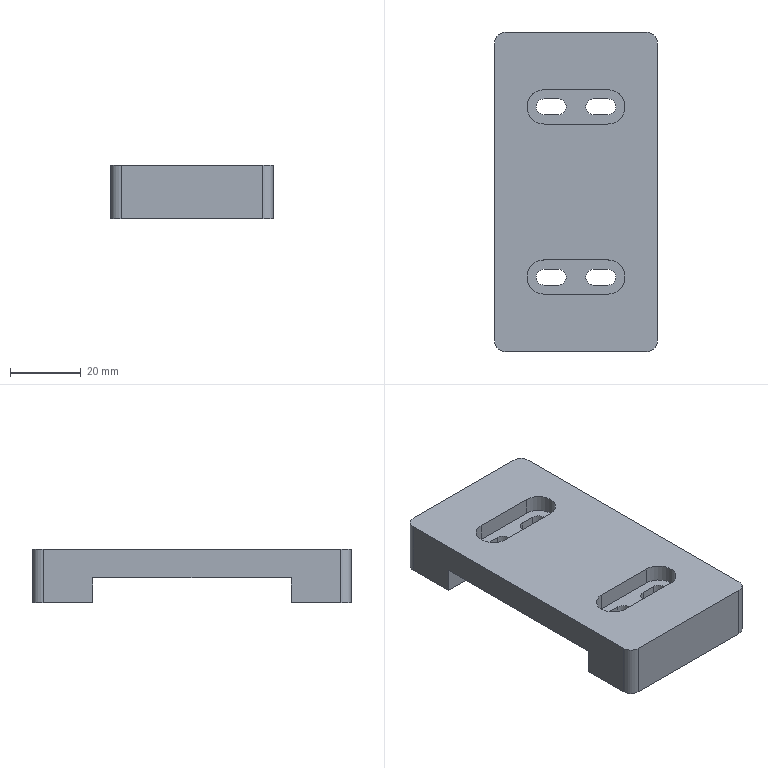Part | STEP file | ROTATION MC_NEW VER-0610_554 | 1 solid | 40 faces | box 46 x 90 x 15 mm | volume 41116 mm3 | plane 24 | cylinder 16 | commonest cylinder face diameters 4.5 x8 6 x4 9.7 x4
STEP:
#1=CARTESIAN_POINT('',(382.531,403.318,-54.091));
#2=VERTEX_POINT('',#1);
#3=CARTESIAN_POINT('',(382.531,403.318,-58.891));
#4=VERTEX_POINT('',#3);
#5=CARTESIAN_POINT('',(382.531,403.318,-54.091));
#6=DIRECTION('',(0.,0.,-1.));
#7=VECTOR('',#6,4.8);
#8=LINE('',#5,#7);
#9=EDGE_CURVE('',#2,#4,#8,.T.);
#10=ORIENTED_EDGE('',*,*,#9,.F.);
#11=CARTESIAN_POINT('',(382.531,393.618,-54.091));
#12=VERTEX_POINT('',#11);
#13=CARTESIAN_POINT('',(382.531,398.468,-54.091));
#14=DIRECTION('',(0.,0.,1.));
#15=DIRECTION('',(-1.,0.,0.));
#16=AXIS2_PLACEMENT_3D('',#13,#14,#15);
#17=CIRCLE('',#16,4.85);
#18=EDGE_CURVE('',#2,#12,#17,.T.);
#19=ORIENTED_EDGE('',*,*,#18,.T.);
#20=CARTESIAN_POINT('',(382.531,393.618,-58.891));
#21=VERTEX_POINT('',#20);
#22=CARTESIAN_POINT('',(382.531,393.618,-58.891));
#23=DIRECTION('',(0.,0.,1.));
#24=VECTOR('',#23,4.8);
#25=LINE('',#22,#24);
#26=EDGE_CURVE('',#21,#12,#25,.T.);
#27=ORIENTED_EDGE('',*,*,#26,.F.);
#28=CARTESIAN_POINT('',(382.531,398.468,-58.891));
#29=DIRECTION('',(0.,0.,-1.));
#30=DIRECTION('',(-1.,0.,0.));
#31=AXIS2_PLACEMENT_3D('',#28,#29,#30);
#32=CIRCLE('',#31,4.85);
#33=EDGE_CURVE('',#21,#4,#32,.T.);
#34=ORIENTED_EDGE('',*,*,#33,.T.);
#35=EDGE_LOOP('',(#10,#19,#27,#34));
#36=FACE_OUTER_BOUND('',#35,.T.);
#37=CARTESIAN_POINT('',(382.531,398.468,-74.091));
#38=DIRECTION('',(0.,0.,1.));
#39=DIRECTION('',(-1.,0.,0.));
#40=AXIS2_PLACEMENT_3D('',#37,#38,#39);
#41=CYLINDRICAL_SURFACE('',#40,4.85);
#42=ADVANCED_FACE('',(#36),#41,.F.);
#43=ORIENTED_EDGE('',*,*,#9,.T.);
#44=CARTESIAN_POINT('',(400.531,403.318,-58.891));
#45=VERTEX_POINT('',#44);
#46=CARTESIAN_POINT('',(382.531,403.318,-58.891));
#47=DIRECTION('',(1.,0.,0.));
#48=VECTOR('',#47,18.);
#49=LINE('',#46,#48);
#50=EDGE_CURVE('',#4,#45,#49,.T.);
#51=ORIENTED_EDGE('',*,*,#50,.T.);
#52=CARTESIAN_POINT('',(400.531,403.318,-54.091));
#53=VERTEX_POINT('',#52);
#54=CARTESIAN_POINT('',(400.531,403.318,-58.891));
#55=DIRECTION('',(0.,0.,1.));
#56=VECTOR('',#55,4.8);
#57=LINE('',#54,#56);
#58=EDGE_CURVE('',#45,#53,#57,.T.);
#59=ORIENTED_EDGE('',*,*,#58,.T.);
#60=CARTESIAN_POINT('',(400.531,403.318,-54.091));
#61=DIRECTION('',(-1.,0.,0.));
#62=VECTOR('',#61,18.);
#63=LINE('',#60,#62);
#64=EDGE_CURVE('',#53,#2,#63,.T.);
#65=ORIENTED_EDGE('',*,*,#64,.T.);
#66=EDGE_LOOP('',(#43,#51,#59,#65));
#67=FACE_OUTER_BOUND('',#66,.T.);
#68=CARTESIAN_POINT('',(384.531,403.318,-74.091));
#69=DIRECTION('',(0.,1.,0.));
#70=DIRECTION('',(0.,0.,1.));
#71=AXIS2_PLACEMENT_3D('',#68,#69,#70);
#72=PLANE('',#71);
#73=ADVANCED_FACE('',(#67),#72,.F.);
#74=ORIENTED_EDGE('',*,*,#26,.T.);
#75=CARTESIAN_POINT('',(400.531,393.618,-54.091));
#76=VERTEX_POINT('',#75);
#77=CARTESIAN_POINT('',(382.531,393.618,-54.091));
#78=DIRECTION('',(1.,0.,0.));
#79=VECTOR('',#78,18.);
#80=LINE('',#77,#79);
#81=EDGE_CURVE('',#12,#76,#80,.T.);
#82=ORIENTED_EDGE('',*,*,#81,.T.);
#83=CARTESIAN_POINT('',(400.531,393.618,-58.891));
#84=VERTEX_POINT('',#83);
#85=CARTESIAN_POINT('',(400.531,393.618,-54.091));
#86=DIRECTION('',(0.,0.,-1.));
#87=VECTOR('',#86,4.8);
#88=LINE('',#85,#87);
#89=EDGE_CURVE('',#76,#84,#88,.T.);
#90=ORIENTED_EDGE('',*,*,#89,.T.);
#91=CARTESIAN_POINT('',(400.531,393.618,-58.891));
#92=DIRECTION('',(-1.,0.,0.));
#93=VECTOR('',#92,18.);
#94=LINE('',#91,#93);
#95=EDGE_CURVE('',#84,#21,#94,.T.);
#96=ORIENTED_EDGE('',*,*,#95,.T.);
#97=EDGE_LOOP('',(#74,#82,#90,#96));
#98=FACE_OUTER_BOUND('',#97,.T.);
#99=CARTESIAN_POINT('',(384.531,393.618,-74.091));
#100=DIRECTION('',(0.,-1.,0.));
#101=DIRECTION('',(0.,0.,-1.));
#102=AXIS2_PLACEMENT_3D('',#99,#100,#101);
#103=PLANE('',#102);
#104=ADVANCED_FACE('',(#98),#103,.F.);
#105=CARTESIAN_POINT('',(382.531,400.718,-58.891));
#106=VERTEX_POINT('',#105);
#107=CARTESIAN_POINT('',(382.531,396.218,-58.891));
#108=VERTEX_POINT('',#107);
#109=CARTESIAN_POINT('',(382.531,398.468,-58.891));
#110=DIRECTION('',(0.,0.,1.));
#111=DIRECTION('',(-1.,0.,0.));
#112=AXIS2_PLACEMENT_3D('',#109,#110,#111);
#113=CIRCLE('',#112,2.25);
#114=EDGE_CURVE('',#106,#108,#113,.T.);
#115=ORIENTED_EDGE('',*,*,#114,.T.);
#116=CARTESIAN_POINT('',(382.531,396.218,-62.091));
#117=VERTEX_POINT('',#116);
#118=CARTESIAN_POINT('',(382.531,396.218,-62.091));
#119=DIRECTION('',(0.,0.,1.));
#120=VECTOR('',#119,3.2);
#121=LINE('',#118,#120);
#122=EDGE_CURVE('',#117,#108,#121,.T.);
#123=ORIENTED_EDGE('',*,*,#122,.F.);
#124=CARTESIAN_POINT('',(382.531,400.718,-62.091));
#125=VERTEX_POINT('',#124);
#126=CARTESIAN_POINT('',(382.531,398.468,-62.091));
#127=DIRECTION('',(0.,0.,1.));
#128=DIRECTION('',(1.,0.,0.));
#129=AXIS2_PLACEMENT_3D('',#126,#127,#128);
#130=CIRCLE('',#129,2.25);
#131=EDGE_CURVE('',#125,#117,#130,.T.);
#132=ORIENTED_EDGE('',*,*,#131,.F.);
#133=CARTESIAN_POINT('',(382.531,400.718,-58.891));
#134=DIRECTION('',(0.,0.,-1.));
#135=VECTOR('',#134,3.2);
#136=LINE('',#133,#135);
#137=EDGE_CURVE('',#106,#125,#136,.T.);
#138=ORIENTED_EDGE('',*,*,#137,.F.);
#139=EDGE_LOOP('',(#115,#123,#132,#138));
#140=FACE_OUTER_BOUND('',#139,.T.);
#141=CARTESIAN_POINT('',(382.531,398.468,-74.091));
#142=DIRECTION('',(0.,0.,1.));
#143=DIRECTION('',(-1.,0.,0.));
#144=AXIS2_PLACEMENT_3D('',#141,#142,#143);
#145=CYLINDRICAL_SURFACE('',#144,2.25);
#146=ADVANCED_FACE('',(#140),#145,.F.);
#147=CARTESIAN_POINT('',(396.531,400.718,-58.891));
#148=VERTEX_POINT('',#147);
#149=CARTESIAN_POINT('',(396.531,396.218,-58.891));
#150=VERTEX_POINT('',#149);
#151=CARTESIAN_POINT('',(396.531,398.468,-58.891));
#152=DIRECTION('',(0.,0.,1.));
#153=DIRECTION('',(-1.,0.,0.));
#154=AXIS2_PLACEMENT_3D('',#151,#152,#153);
#155=CIRCLE('',#154,2.25);
#156=EDGE_CURVE('',#148,#150,#155,.T.);
#157=ORIENTED_EDGE('',*,*,#156,.T.);
#158=CARTESIAN_POINT('',(396.531,396.218,-62.091));
#159=VERTEX_POINT('',#158);
#160=CARTESIAN_POINT('',(396.531,396.218,-62.091));
#161=DIRECTION('',(0.,0.,1.));
#162=VECTOR('',#161,3.2);
#163=LINE('',#160,#162);
#164=EDGE_CURVE('',#159,#150,#163,.T.);
#165=ORIENTED_EDGE('',*,*,#164,.F.);
#166=CARTESIAN_POINT('',(396.531,400.718,-62.091));
#167=VERTEX_POINT('',#166);
#168=CARTESIAN_POINT('',(396.531,398.468,-62.091));
#169=DIRECTION('',(0.,0.,-1.));
#170=DIRECTION('',(1.,0.,0.));
#171=AXIS2_PLACEMENT_3D('',#168,#169,#170);
#172=CIRCLE('',#171,2.25);
#173=EDGE_CURVE('',#159,#167,#172,.T.);
#174=ORIENTED_EDGE('',*,*,#173,.T.);
#175=CARTESIAN_POINT('',(396.531,400.718,-58.891));
#176=DIRECTION('',(0.,0.,-1.));
#177=VECTOR('',#176,3.2);
#178=LINE('',#175,#177);
#179=EDGE_CURVE('',#148,#167,#178,.T.);
#180=ORIENTED_EDGE('',*,*,#179,.F.);
#181=EDGE_LOOP('',(#157,#165,#174,#180));
#182=FACE_OUTER_BOUND('',#181,.T.);
#183=CARTESIAN_POINT('',(396.531,398.468,-74.091));
#184=DIRECTION('',(0.,0.,1.));
#185=DIRECTION('',(-1.,0.,0.));
#186=AXIS2_PLACEMENT_3D('',#183,#184,#185);
#187=CYLINDRICAL_SURFACE('',#186,2.25);
#188=ADVANCED_FACE('',(#182),#187,.F.);
#189=CARTESIAN_POINT('',(386.531,396.218,-58.891));
#190=VERTEX_POINT('',#189);
#191=CARTESIAN_POINT('',(386.531,400.718,-58.891));
#192=VERTEX_POINT('',#191);
#193=CARTESIAN_POINT('',(386.531,398.468,-58.891));
#194=DIRECTION('',(0.,0.,1.));
#195=DIRECTION('',(-1.,0.,0.));
#196=AXIS2_PLACEMENT_3D('',#193,#194,#195);
#197=CIRCLE('',#196,2.25);
#198=EDGE_CURVE('',#190,#192,#197,.T.);
#199=ORIENTED_EDGE('',*,*,#198,.T.);
#200=CARTESIAN_POINT('',(386.531,400.718,-62.091));
#201=VERTEX_POINT('',#200);
#202=CARTESIAN_POINT('',(386.531,400.718,-62.091));
#203=DIRECTION('',(0.,0.,1.));
#204=VECTOR('',#203,3.2);
#205=LINE('',#202,#204);
#206=EDGE_CURVE('',#201,#192,#205,.T.);
#207=ORIENTED_EDGE('',*,*,#206,.F.);
#208=CARTESIAN_POINT('',(386.531,396.218,-62.091));
#209=VERTEX_POINT('',#208);
#210=CARTESIAN_POINT('',(386.531,398.468,-62.091));
#211=DIRECTION('',(0.,0.,-1.));
#212=DIRECTION('',(1.,0.,0.));
#213=AXIS2_PLACEMENT_3D('',#210,#211,#212);
#214=CIRCLE('',#213,2.25);
#215=EDGE_CURVE('',#201,#209,#214,.T.);
#216=ORIENTED_EDGE('',*,*,#215,.T.);
#217=CARTESIAN_POINT('',(386.531,396.218,-58.891));
#218=DIRECTION('',(0.,0.,-1.));
#219=VECTOR('',#218,3.2);
#220=LINE('',#217,#219);
#221=EDGE_CURVE('',#190,#209,#220,.T.);
#222=ORIENTED_EDGE('',*,*,#221,.F.);
#223=EDGE_LOOP('',(#199,#207,#216,#222));
#224=FACE_OUTER_BOUND('',#223,.T.);
#225=CARTESIAN_POINT('',(386.531,398.468,-74.091));
#226=DIRECTION('',(0.,0.,1.));
#227=DIRECTION('',(1.,0.,0.));
#228=AXIS2_PLACEMENT_3D('',#225,#226,#227);
#229=CYLINDRICAL_SURFACE('',#228,2.25);
#230=ADVANCED_FACE('',(#224),#229,.F.);
#231=ORIENTED_EDGE('',*,*,#95,.F.);
#232=CARTESIAN_POINT('',(400.531,398.468,-58.891));
#233=DIRECTION('',(0.,0.,-1.));
#234=DIRECTION('',(-1.,0.,0.));
#235=AXIS2_PLACEMENT_3D('',#232,#233,#234);
#236=CIRCLE('',#235,4.85);
#237=EDGE_CURVE('',#45,#84,#236,.T.);
#238=ORIENTED_EDGE('',*,*,#237,.F.);
#239=ORIENTED_EDGE('',*,*,#50,.F.);
#240=ORIENTED_EDGE('',*,*,#33,.F.);
#241=EDGE_LOOP('',(#231,#238,#239,#240));
#242=FACE_OUTER_BOUND('',#241,.T.);
#243=CARTESIAN_POINT('',(382.531,396.218,-58.891));
#244=DIRECTION('',(1.,0.,0.));
#245=VECTOR('',#244,4.);
#246=LINE('',#243,#245);
#247=EDGE_CURVE('',#108,#190,#246,.T.);
#248=ORIENTED_EDGE('',*,*,#247,.F.);
#249=ORIENTED_EDGE('',*,*,#114,.F.);
#250=CARTESIAN_POINT('',(386.531,400.718,-58.891));
#251=DIRECTION('',(-1.,0.,0.));
#252=VECTOR('',#251,4.);
#253=LINE('',#250,#252);
#254=EDGE_CURVE('',#192,#106,#253,.T.);
#255=ORIENTED_EDGE('',*,*,#254,.F.);
#256=ORIENTED_EDGE('',*,*,#198,.F.);
#257=EDGE_LOOP('',(#248,#249,#255,#256));
#258=FACE_BOUND('',#257,.T.);
#259=CARTESIAN_POINT('',(400.531,396.218,-58.891));
#260=VERTEX_POINT('',#259);
#261=CARTESIAN_POINT('',(396.531,396.218,-58.891));
#262=DIRECTION('',(1.,0.,0.));
#263=VECTOR('',#262,4.);
#264=LINE('',#261,#263);
#265=EDGE_CURVE('',#150,#260,#264,.T.);
#266=ORIENTED_EDGE('',*,*,#265,.F.);
#267=ORIENTED_EDGE('',*,*,#156,.F.);
#268=CARTESIAN_POINT('',(400.531,400.718,-58.891));
#269=VERTEX_POINT('',#268);
#270=CARTESIAN_POINT('',(400.531,400.718,-58.891));
#271=DIRECTION('',(-1.,0.,0.));
#272=VECTOR('',#271,4.);
#273=LINE('',#270,#272);
#274=EDGE_CURVE('',#269,#148,#273,.T.);
#275=ORIENTED_EDGE('',*,*,#274,.F.);
#276=CARTESIAN_POINT('',(400.531,398.468,-58.891));
#277=DIRECTION('',(0.,0.,1.));
#278=DIRECTION('',(-1.,0.,0.));
#279=AXIS2_PLACEMENT_3D('',#276,#277,#278);
#280=CIRCLE('',#279,2.25);
#281=EDGE_CURVE('',#260,#269,#280,.T.);
#282=ORIENTED_EDGE('',*,*,#281,.F.);
#283=EDGE_LOOP('',(#266,#267,#275,#282));
#284=FACE_BOUND('',#283,.T.);
#285=CARTESIAN_POINT('',(391.531,422.468,-58.891));
#286=DIRECTION('',(0.,0.,1.));
#287=DIRECTION('',(1.,0.,0.));
#288=AXIS2_PLACEMENT_3D('',#285,#286,#287);
#289=PLANE('',#288);
#290=ADVANCED_FACE('',(#242,#258,#284),#289,.T.);
#291=ORIENTED_EDGE('',*,*,#254,.T.);
#292=ORIENTED_EDGE('',*,*,#137,.T.);
#293=CARTESIAN_POINT('',(382.531,400.718,-62.091));
#294=DIRECTION('',(1.,0.,0.));
#295=VECTOR('',#294,4.);
#296=LINE('',#293,#295);
#297=EDGE_CURVE('',#125,#201,#296,.T.);
#298=ORIENTED_EDGE('',*,*,#297,.T.);
#299=ORIENTED_EDGE('',*,*,#206,.T.);
#300=EDGE_LOOP('',(#291,#292,#298,#299));
#301=FACE_OUTER_BOUND('',#300,.T.);
#302=CARTESIAN_POINT('',(384.531,400.718,-74.091));
#303=DIRECTION('',(0.,1.,0.));
#304=DIRECTION('',(0.,0.,1.));
#305=AXIS2_PLACEMENT_3D('',#302,#303,#304);
#306=PLANE('',#305);
#307=ADVANCED_FACE('',(#301),#306,.F.);
#308=ORIENTED_EDGE('',*,*,#247,.T.);
#309=ORIENTED_EDGE('',*,*,#221,.T.);
#310=CARTESIAN_POINT('',(386.531,396.218,-62.091));
#311=DIRECTION('',(-1.,0.,0.));
#312=VECTOR('',#311,4.);
#313=LINE('',#310,#312);
#314=EDGE_CURVE('',#209,#117,#313,.T.);
#315=ORIENTED_EDGE('',*,*,#314,.T.);
#316=ORIENTED_EDGE('',*,*,#122,.T.);
#317=EDGE_LOOP('',(#308,#309,#315,#316));
#318=FACE_OUTER_BOUND('',#317,.T.);
#319=CARTESIAN_POINT('',(384.531,396.218,-74.091));
#320=DIRECTION('',(0.,-1.,0.));
#321=DIRECTION('',(0.,0.,-1.));
#322=AXIS2_PLACEMENT_3D('',#319,#320,#321);
#323=PLANE('',#322);
#324=ADVANCED_FACE('',(#318),#323,.F.);
#325=ORIENTED_EDGE('',*,*,#265,.T.);
#326=CARTESIAN_POINT('',(400.531,396.218,-62.091));
#327=VERTEX_POINT('',#326);
#328=CARTESIAN_POINT('',(400.531,396.218,-58.891));
#329=DIRECTION('',(0.,0.,-1.));
#330=VECTOR('',#329,3.2);
#331=LINE('',#328,#330);
#332=EDGE_CURVE('',#260,#327,#331,.T.);
#333=ORIENTED_EDGE('',*,*,#332,.T.);
#334=CARTESIAN_POINT('',(400.531,396.218,-62.091));
#335=DIRECTION('',(-1.,0.,0.));
#336=VECTOR('',#335,4.);
#337=LINE('',#334,#336);
#338=EDGE_CURVE('',#327,#159,#337,.T.);
#339=ORIENTED_EDGE('',*,*,#338,.T.);
#340=ORIENTED_EDGE('',*,*,#164,.T.);
#341=EDGE_LOOP('',(#325,#333,#339,#340));
#342=FACE_OUTER_BOUND('',#341,.T.);
#343=CARTESIAN_POINT('',(398.531,396.218,-74.091));
#344=DIRECTION('',(0.,-1.,0.));
#345=DIRECTION('',(0.,0.,-1.));
#346=AXIS2_PLACEMENT_3D('',#343,#344,#345);
#347=PLANE('',#346);
#348=ADVANCED_FACE('',(#342),#347,.F.);
#349=ORIENTED_EDGE('',*,*,#274,.T.);
#350=ORIENTED_EDGE('',*,*,#179,.T.);
#351=CARTESIAN_POINT('',(400.531,400.718,-62.091));
#352=VERTEX_POINT('',#351);
#353=CARTESIAN_POINT('',(396.531,400.718,-62.091));
#354=DIRECTION('',(1.,0.,0.));
#355=VECTOR('',#354,4.);
#356=LINE('',#353,#355);
#357=EDGE_CURVE('',#167,#352,#356,.T.);
#358=ORIENTED_EDGE('',*,*,#357,.T.);
#359=CARTESIAN_POINT('',(400.531,400.718,-62.091));
#360=DIRECTION('',(0.,0.,1.));
#361=VECTOR('',#360,3.2);
#362=LINE('',#359,#361);
#363=EDGE_CURVE('',#352,#269,#362,.T.);
#364=ORIENTED_EDGE('',*,*,#363,.T.);
#365=EDGE_LOOP('',(#349,#350,#358,#364));
#366=FACE_OUTER_BOUND('',#365,.T.);
#367=CARTESIAN_POINT('',(398.531,400.718,-74.091));
#368=DIRECTION('',(0.,1.,0.));
#369=DIRECTION('',(0.,0.,1.));
#370=AXIS2_PLACEMENT_3D('',#367,#368,#369);
#371=PLANE('',#370);
#372=ADVANCED_FACE('',(#366),#371,.F.);
#373=ORIENTED_EDGE('',*,*,#281,.T.);
#374=ORIENTED_EDGE('',*,*,#363,.F.);
#375=CARTESIAN_POINT('',(400.531,398.468,-62.091));
#376=DIRECTION('',(0.,0.,-1.));
#377=DIRECTION('',(1.,0.,0.));
#378=AXIS2_PLACEMENT_3D('',#375,#376,#377);
#379=CIRCLE('',#378,2.25);
#380=EDGE_CURVE('',#352,#327,#379,.T.);
#381=ORIENTED_EDGE('',*,*,#380,.T.);
#382=ORIENTED_EDGE('',*,*,#332,.F.);
#383=EDGE_LOOP('',(#373,#374,#381,#382));
#384=FACE_OUTER_BOUND('',#383,.T.);
#385=CARTESIAN_POINT('',(400.531,398.468,-74.091));
#386=DIRECTION('',(0.,0.,1.));
#387=DIRECTION('',(1.,0.,0.));
#388=AXIS2_PLACEMENT_3D('',#385,#386,#387);
#389=CYLINDRICAL_SURFACE('',#388,2.25);
#390=ADVANCED_FACE('',(#384),#389,.F.);
#391=ORIENTED_EDGE('',*,*,#89,.F.);
#392=CARTESIAN_POINT('',(400.531,398.468,-54.091));
#393=DIRECTION('',(0.,0.,1.));
#394=DIRECTION('',(-1.,0.,0.));
#395=AXIS2_PLACEMENT_3D('',#392,#393,#394);
#396=CIRCLE('',#395,4.85);
#397=EDGE_CURVE('',#76,#53,#396,.T.);
#398=ORIENTED_EDGE('',*,*,#397,.T.);
#399=ORIENTED_EDGE('',*,*,#58,.F.);
#400=ORIENTED_EDGE('',*,*,#237,.T.);
#401=EDGE_LOOP('',(#391,#398,#399,#400));
#402=FACE_OUTER_BOUND('',#401,.T.);
#403=CARTESIAN_POINT('',(400.531,398.468,-74.091));
#404=DIRECTION('',(0.,0.,1.));
#405=DIRECTION('',(1.,0.,0.));
#406=AXIS2_PLACEMENT_3D('',#403,#404,#405);
#407=CYLINDRICAL_SURFACE('',#406,4.85);
#408=ADVANCED_FACE('',(#402),#407,.F.);
#409=CARTESIAN_POINT('',(368.531,380.468,-54.091));
#410=VERTEX_POINT('',#409);
#411=CARTESIAN_POINT('',(371.531,377.468,-54.091));
#412=VERTEX_POINT('',#411);
#413=CARTESIAN_POINT('',(371.531,380.468,-54.091));
#414=DIRECTION('',(0.,0.,1.));
#415=DIRECTION('',(-0.7071,-0.7071,0.));
#416=AXIS2_PLACEMENT_3D('',#413,#414,#415);
#417=CIRCLE('',#416,3.);
#418=EDGE_CURVE('',#410,#412,#417,.T.);
#419=ORIENTED_EDGE('',*,*,#418,.T.);
#420=CARTESIAN_POINT('',(411.531,377.468,-54.091));
#421=VERTEX_POINT('',#420);
#422=CARTESIAN_POINT('',(371.531,377.468,-54.091));
#423=DIRECTION('',(1.,0.,0.));
#424=VECTOR('',#423,40.);
#425=LINE('',#422,#424);
#426=EDGE_CURVE('',#412,#421,#425,.T.);
#427=ORIENTED_EDGE('',*,*,#426,.T.);
#428=CARTESIAN_POINT('',(414.531,380.468,-54.091));
#429=VERTEX_POINT('',#428);
#430=CARTESIAN_POINT('',(411.531,380.468,-54.091));
#431=DIRECTION('',(0.,0.,1.));
#432=DIRECTION('',(0.,-1.,0.));
#433=AXIS2_PLACEMENT_3D('',#430,#431,#432);
#434=CIRCLE('',#433,3.);
#435=EDGE_CURVE('',#421,#429,#434,.T.);
#436=ORIENTED_EDGE('',*,*,#435,.T.);
#437=CARTESIAN_POINT('',(414.531,464.468,-54.091));
#438=VERTEX_POINT('',#437);
#439=CARTESIAN_POINT('',(414.531,380.468,-54.091));
#440=DIRECTION('',(0.,1.,0.));
#441=VECTOR('',#440,84.);
#442=LINE('',#439,#441);
#443=EDGE_CURVE('',#429,#438,#442,.T.);
#444=ORIENTED_EDGE('',*,*,#443,.T.);
#445=CARTESIAN_POINT('',(411.531,467.468,-54.091));
#446=VERTEX_POINT('',#445);
#447=CARTESIAN_POINT('',(411.531,464.468,-54.091));
#448=DIRECTION('',(0.,0.,1.));
#449=DIRECTION('',(1.,0.,0.));
#450=AXIS2_PLACEMENT_3D('',#447,#448,#449);
#451=CIRCLE('',#450,3.);
#452=EDGE_CURVE('',#438,#446,#451,.T.);
#453=ORIENTED_EDGE('',*,*,#452,.T.);
#454=CARTESIAN_POINT('',(371.531,467.468,-54.091));
#455=VERTEX_POINT('',#454);
#456=CARTESIAN_POINT('',(411.531,467.468,-54.091));
#457=DIRECTION('',(-1.,0.,0.));
#458=VECTOR('',#457,40.);
#459=LINE('',#456,#458);
#460=EDGE_CURVE('',#446,#455,#459,.T.);
#461=ORIENTED_EDGE('',*,*,#460,.T.);
#462=CARTESIAN_POINT('',(368.531,464.468,-54.091));
#463=VERTEX_POINT('',#462);
#464=CARTESIAN_POINT('',(371.531,464.468,-54.091));
#465=DIRECTION('',(0.,0.,1.));
#466=DIRECTION('',(0.,1.,0.));
#467=AXIS2_PLACEMENT_3D('',#464,#465,#466);
#468=CIRCLE('',#467,3.);
#469=EDGE_CURVE('',#455,#463,#468,.T.);
#470=ORIENTED_EDGE('',*,*,#469,.T.);
#471=CARTESIAN_POINT('',(368.531,464.468,-54.091));
#472=DIRECTION('',(0.,-1.,0.));
#473=VECTOR('',#472,84.);
#474=LINE('',#471,#473);
#475=EDGE_CURVE('',#463,#410,#474,.T.);
#476=ORIENTED_EDGE('',*,*,#475,.T.);
#477=EDGE_LOOP('',(#419,#427,#436,#444,#453,#461,#470,#476));
#478=FACE_OUTER_BOUND('',#477,.T.);
#479=CARTESIAN_POINT('',(382.531,441.618,-54.091));
#480=VERTEX_POINT('',#479);
#481=CARTESIAN_POINT('',(400.531,441.618,-54.091));
#482=VERTEX_POINT('',#481);
#483=CARTESIAN_POINT('',(382.531,441.618,-54.091));
#484=DIRECTION('',(1.,0.,0.));
#485=VECTOR('',#484,18.);
#486=LINE('',#483,#485);
#487=EDGE_CURVE('',#480,#482,#486,.T.);
#488=ORIENTED_EDGE('',*,*,#487,.F.);
#489=CARTESIAN_POINT('',(382.531,451.318,-54.091));
#490=VERTEX_POINT('',#489);
#491=CARTESIAN_POINT('',(382.531,446.468,-54.091));
#492=DIRECTION('',(0.,0.,-1.));
#493=DIRECTION('',(-1.,0.,0.));
#494=AXIS2_PLACEMENT_3D('',#491,#492,#493);
#495=CIRCLE('',#494,4.85);
#496=EDGE_CURVE('',#480,#490,#495,.T.);
#497=ORIENTED_EDGE('',*,*,#496,.T.);
#498=CARTESIAN_POINT('',(400.531,451.318,-54.091));
#499=VERTEX_POINT('',#498);
#500=CARTESIAN_POINT('',(400.531,451.318,-54.091));
#501=DIRECTION('',(-1.,0.,0.));
#502=VECTOR('',#501,18.);
#503=LINE('',#500,#502);
#504=EDGE_CURVE('',#499,#490,#503,.T.);
#505=ORIENTED_EDGE('',*,*,#504,.F.);
#506=CARTESIAN_POINT('',(400.531,446.468,-54.091));
#507=DIRECTION('',(0.,0.,-1.));
#508=DIRECTION('',(-1.,0.,0.));
#509=AXIS2_PLACEMENT_3D('',#506,#507,#508);
#510=CIRCLE('',#509,4.85);
#511=EDGE_CURVE('',#499,#482,#510,.T.);
#512=ORIENTED_EDGE('',*,*,#511,.T.);
#513=EDGE_LOOP('',(#488,#497,#505,#512));
#514=FACE_BOUND('',#513,.T.);
#515=ORIENTED_EDGE('',*,*,#397,.F.);
#516=ORIENTED_EDGE('',*,*,#81,.F.);
#517=ORIENTED_EDGE('',*,*,#18,.F.);
#518=ORIENTED_EDGE('',*,*,#64,.F.);
#519=EDGE_LOOP('',(#515,#516,#517,#518));
#520=FACE_BOUND('',#519,.T.);
#521=CARTESIAN_POINT('',(389.531,422.468,-54.091));
#522=DIRECTION('',(0.,0.,1.));
#523=DIRECTION('',(1.,0.,0.));
#524=AXIS2_PLACEMENT_3D('',#521,#522,#523);
#525=PLANE('',#524);
#526=ADVANCED_FACE('',(#478,#514,#520),#525,.T.);
#527=CARTESIAN_POINT('',(382.531,441.618,-58.891));
#528=VERTEX_POINT('',#527);
#529=CARTESIAN_POINT('',(382.531,441.618,-58.891));
#530=DIRECTION('',(0.,0.,1.));
#531=VECTOR('',#530,4.8);
#532=LINE('',#529,#531);
#533=EDGE_CURVE('',#528,#480,#532,.T.);
#534=ORIENTED_EDGE('',*,*,#533,.T.);
#535=ORIENTED_EDGE('',*,*,#487,.T.);
#536=CARTESIAN_POINT('',(400.531,441.618,-58.891));
#537=VERTEX_POINT('',#536);
#538=CARTESIAN_POINT('',(400.531,441.618,-54.091));
#539=DIRECTION('',(0.,0.,-1.));
#540=VECTOR('',#539,4.8);
#541=LINE('',#538,#540);
#542=EDGE_CURVE('',#482,#537,#541,.T.);
#543=ORIENTED_EDGE('',*,*,#542,.T.);
#544=CARTESIAN_POINT('',(400.531,441.618,-58.891));
#545=DIRECTION('',(-1.,0.,0.));
#546=VECTOR('',#545,18.);
#547=LINE('',#544,#546);
#548=EDGE_CURVE('',#537,#528,#547,.T.);
#549=ORIENTED_EDGE('',*,*,#548,.T.);
#550=EDGE_LOOP('',(#534,#535,#543,#549));
#551=FACE_OUTER_BOUND('',#550,.T.);
#552=CARTESIAN_POINT('',(384.531,441.618,-74.091));
#553=DIRECTION('',(0.,-1.,0.));
#554=DIRECTION('',(0.,0.,-1.));
#555=AXIS2_PLACEMENT_3D('',#552,#553,#554);
#556=PLANE('',#555);
#557=ADVANCED_FACE('',(#551),#556,.F.);
#558=ORIENTED_EDGE('',*,*,#533,.F.);
#559=CARTESIAN_POINT('',(382.531,451.318,-58.891));
#560=VERTEX_POINT('',#559);
#561=CARTESIAN_POINT('',(382.531,446.468,-58.891));
#562=DIRECTION('',(0.,0.,-1.));
#563=DIRECTION('',(-1.,0.,0.));
#564=AXIS2_PLACEMENT_3D('',#561,#562,#563);
#565=CIRCLE('',#564,4.85);
#566=EDGE_CURVE('',#528,#560,#565,.T.);
#567=ORIENTED_EDGE('',*,*,#566,.T.);
#568=CARTESIAN_POINT('',(382.531,451.318,-54.091));
#569=DIRECTION('',(0.,0.,-1.));
#570=VECTOR('',#569,4.8);
#571=LINE('',#568,#570);
#572=EDGE_CURVE('',#490,#560,#571,.T.);
#573=ORIENTED_EDGE('',*,*,#572,.F.);
#574=ORIENTED_EDGE('',*,*,#496,.F.);
#575=EDGE_LOOP('',(#558,#567,#573,#574));
#576=FACE_OUTER_BOUND('',#575,.T.);
#577=CARTESIAN_POINT('',(382.531,446.468,-74.091));
#578=DIRECTION('',(0.,0.,1.));
#579=DIRECTION('',(-1.,0.,0.));
#580=AXIS2_PLACEMENT_3D('',#577,#578,#579);
#581=CYLINDRICAL_SURFACE('',#580,4.85);
#582=ADVANCED_FACE('',(#576),#581,.F.);
#583=ORIENTED_EDGE('',*,*,#572,.T.);
#584=CARTESIAN_POINT('',(400.531,451.318,-58.891));
#585=VERTEX_POINT('',#584);
#586=CARTESIAN_POINT('',(382.531,451.318,-58.891));
#587=DIRECTION('',(1.,0.,0.));
#588=VECTOR('',#587,18.);
#589=LINE('',#586,#588);
#590=EDGE_CURVE('',#560,#585,#589,.T.);
#591=ORIENTED_EDGE('',*,*,#590,.T.);
#592=CARTESIAN_POINT('',(400.531,451.318,-58.891));
#593=DIRECTION('',(0.,0.,1.));
#594=VECTOR('',#593,4.8);
#595=LINE('',#592,#594);
#596=EDGE_CURVE('',#585,#499,#595,.T.);
#597=ORIENTED_EDGE('',*,*,#596,.T.);
#598=ORIENTED_EDGE('',*,*,#504,.T.);
#599=EDGE_LOOP('',(#583,#591,#597,#598));
#600=FACE_OUTER_BOUND('',#599,.T.);
#601=CARTESIAN_POINT('',(384.531,451.318,-74.091));
#602=DIRECTION('',(0.,1.,0.));
#603=DIRECTION('',(0.,0.,1.));
#604=AXIS2_PLACEMENT_3D('',#601,#602,#603);
#605=PLANE('',#604);
#606=ADVANCED_FACE('',(#600),#605,.F.);
#607=ORIENTED_EDGE('',*,*,#596,.F.);
#608=CARTESIAN_POINT('',(400.531,446.468,-58.891));
#609=DIRECTION('',(0.,0.,-1.));
#610=DIRECTION('',(-1.,0.,0.));
#611=AXIS2_PLACEMENT_3D('',#608,#609,#610);
#612=CIRCLE('',#611,4.85);
#613=EDGE_CURVE('',#585,#537,#612,.T.);
#614=ORIENTED_EDGE('',*,*,#613,.T.);
#615=ORIENTED_EDGE('',*,*,#542,.F.);
#616=ORIENTED_EDGE('',*,*,#511,.F.);
#617=EDGE_LOOP('',(#607,#614,#615,#616));
#618=FACE_OUTER_BOUND('',#617,.T.);
#619=CARTESIAN_POINT('',(400.531,446.468,-74.091));
#620=DIRECTION('',(0.,0.,1.));
#621=DIRECTION('',(1.,0.,0.));
#622=AXIS2_PLACEMENT_3D('',#619,#620,#621);
#623=CYLINDRICAL_SURFACE('',#622,4.85);
#624=ADVANCED_FACE('',(#618),#623,.F.);
#625=CARTESIAN_POINT('',(368.531,380.468,-69.091));
#626=VERTEX_POINT('',#625);
#627=CARTESIAN_POINT('',(368.531,380.468,-54.091));
#628=DIRECTION('',(0.,0.,-1.));
#629=VECTOR('',#628,15.);
#630=LINE('',#627,#629);
#631=EDGE_CURVE('',#410,#626,#630,.T.);
#632=ORIENTED_EDGE('',*,*,#631,.T.);
#633=CARTESIAN_POINT('',(371.531,377.468,-69.091));
#634=VERTEX_POINT('',#633);
#635=CARTESIAN_POINT('',(371.531,380.468,-69.091));
#636=DIRECTION('',(0.,0.,-1.));
#637=DIRECTION('',(0.,-1.,0.));
#638=AXIS2_PLACEMENT_3D('',#635,#636,#637);
#639=CIRCLE('',#638,3.);
#640=EDGE_CURVE('',#634,#626,#639,.T.);
#641=ORIENTED_EDGE('',*,*,#640,.F.);
#642=CARTESIAN_POINT('',(371.531,377.468,-69.091));
#643=DIRECTION('',(0.,0.,1.));
#644=VECTOR('',#643,15.);
#645=LINE('',#642,#644);
#646=EDGE_CURVE('',#634,#412,#645,.T.);
#647=ORIENTED_EDGE('',*,*,#646,.T.);
#648=ORIENTED_EDGE('',*,*,#418,.F.);
#649=EDGE_LOOP('',(#632,#641,#647,#648));
#650=FACE_OUTER_BOUND('',#649,.T.);
#651=CARTESIAN_POINT('',(371.531,380.468,-67.091));
#652=DIRECTION('',(0.,0.,-1.));
#653=DIRECTION('',(-0.7071,-0.7071,0.));
#654=AXIS2_PLACEMENT_3D('',#651,#652,#653);
#655=CYLINDRICAL_SURFACE('',#654,3.);
#656=ADVANCED_FACE('',(#650),#655,.T.);
#657=ORIENTED_EDGE('',*,*,#646,.F.);
#658=CARTESIAN_POINT('',(411.531,377.468,-69.091));
#659=VERTEX_POINT('',#658);
#660=CARTESIAN_POINT('',(371.531,377.468,-69.091));
#661=DIRECTION('',(1.,0.,0.));
#662=VECTOR('',#661,40.);
#663=LINE('',#660,#662);
#664=EDGE_CURVE('',#634,#659,#663,.T.);
#665=ORIENTED_EDGE('',*,*,#664,.T.);
#666=CARTESIAN_POINT('',(411.531,377.468,-54.091));
#667=DIRECTION('',(0.,0.,-1.));
#668=VECTOR('',#667,15.);
#669=LINE('',#666,#668);
#670=EDGE_CURVE('',#421,#659,#669,.T.);
#671=ORIENTED_EDGE('',*,*,#670,.F.);
#672=ORIENTED_EDGE('',*,*,#426,.F.);
#673=EDGE_LOOP('',(#657,#665,#671,#672));
#674=FACE_OUTER_BOUND('',#673,.T.);
#675=CARTESIAN_POINT('',(390.531,377.468,-67.091));
#676=DIRECTION('',(0.,-1.,0.));
#677=DIRECTION('',(0.,0.,-1.));
#678=AXIS2_PLACEMENT_3D('',#675,#676,#677);
#679=PLANE('',#678);
#680=ADVANCED_FACE('',(#674),#679,.T.);
#681=ORIENTED_EDGE('',*,*,#670,.T.);
#682=CARTESIAN_POINT('',(414.531,380.468,-69.091));
#683=VERTEX_POINT('',#682);
#684=CARTESIAN_POINT('',(411.531,380.468,-69.091));
#685=DIRECTION('',(0.,0.,-1.));
#686=DIRECTION('',(1.,0.,0.));
#687=AXIS2_PLACEMENT_3D('',#684,#685,#686);
#688=CIRCLE('',#687,3.);
#689=EDGE_CURVE('',#683,#659,#688,.T.);
#690=ORIENTED_EDGE('',*,*,#689,.F.);
#691=CARTESIAN_POINT('',(414.531,380.468,-69.091));
#692=DIRECTION('',(0.,0.,1.));
#693=VECTOR('',#692,15.);
#694=LINE('',#691,#693);
#695=EDGE_CURVE('',#683,#429,#694,.T.);
#696=ORIENTED_EDGE('',*,*,#695,.T.);
#697=ORIENTED_EDGE('',*,*,#435,.F.);
#698=EDGE_LOOP('',(#681,#690,#696,#697));
#699=FACE_OUTER_BOUND('',#698,.T.);
#700=CARTESIAN_POINT('',(411.531,380.468,-67.091));
#701=DIRECTION('',(0.,0.,-1.));
#702=DIRECTION('',(0.7071,-0.7071,0.));
#703=AXIS2_PLACEMENT_3D('',#700,#701,#702);
#704=CYLINDRICAL_SURFACE('',#703,3.);
#705=ADVANCED_FACE('',(#699),#704,.T.);
#706=CARTESIAN_POINT('',(368.531,450.493,-62.091));
#707=VERTEX_POINT('',#706);
#708=CARTESIAN_POINT('',(368.531,394.443,-62.091));
#709=VERTEX_POINT('',#708);
#710=CARTESIAN_POINT('',(368.531,450.493,-62.091));
#711=DIRECTION('',(0.,-1.,0.));
#712=VECTOR('',#711,56.05);
#713=LINE('',#710,#712);
#714=EDGE_CURVE('',#707,#709,#713,.T.);
#715=ORIENTED_EDGE('',*,*,#714,.F.);
#716=CARTESIAN_POINT('',(414.531,450.493,-62.091));
#717=VERTEX_POINT('',#716);
#718=CARTESIAN_POINT('',(414.531,450.493,-62.091));
#719=DIRECTION('',(-1.,0.,0.));
#720=VECTOR('',#719,46.);
#721=LINE('',#718,#720);
#722=EDGE_CURVE('',#717,#707,#721,.T.);
#723=ORIENTED_EDGE('',*,*,#722,.F.);
#724=CARTESIAN_POINT('',(414.531,394.443,-62.091));
#725=VERTEX_POINT('',#724);
#726=CARTESIAN_POINT('',(414.531,394.443,-62.091));
#727=DIRECTION('',(0.,1.,0.));
#728=VECTOR('',#727,56.05);
#729=LINE('',#726,#728);
#730=EDGE_CURVE('',#725,#717,#729,.T.);
#731=ORIENTED_EDGE('',*,*,#730,.F.);
#732=CARTESIAN_POINT('',(368.531,394.443,-62.091));
#733=DIRECTION('',(1.,0.,0.));
#734=VECTOR('',#733,46.);
#735=LINE('',#732,#734);
#736=EDGE_CURVE('',#709,#725,#735,.T.);
#737=ORIENTED_EDGE('',*,*,#736,.F.);
#738=EDGE_LOOP('',(#715,#723,#731,#737));
#739=FACE_OUTER_BOUND('',#738,.T.);
#740=CARTESIAN_POINT('',(400.531,444.218,-62.091));
#741=VERTEX_POINT('',#740);
#742=CARTESIAN_POINT('',(400.531,448.718,-62.091));
#743=VERTEX_POINT('',#742);
#744=CARTESIAN_POINT('',(400.531,446.468,-62.091));
#745=DIRECTION('',(0.,0.,1.));
#746=DIRECTION('',(1.,0.,0.));
#747=AXIS2_PLACEMENT_3D('',#744,#745,#746);
#748=CIRCLE('',#747,2.25);
#749=EDGE_CURVE('',#741,#743,#748,.T.);
#750=ORIENTED_EDGE('',*,*,#749,.T.);
#751=CARTESIAN_POINT('',(396.531,448.718,-62.091));
#752=VERTEX_POINT('',#751);
#753=CARTESIAN_POINT('',(396.531,448.718,-62.091));
#754=DIRECTION('',(1.,0.,0.));
#755=VECTOR('',#754,4.);
#756=LINE('',#753,#755);
#757=EDGE_CURVE('',#752,#743,#756,.T.);
#758=ORIENTED_EDGE('',*,*,#757,.F.);
#759=CARTESIAN_POINT('',(396.531,444.218,-62.091));
#760=VERTEX_POINT('',#759);
#761=CARTESIAN_POINT('',(396.531,446.468,-62.091));
#762=DIRECTION('',(0.,0.,1.));
#763=DIRECTION('',(1.,0.,0.));
#764=AXIS2_PLACEMENT_3D('',#761,#762,#763);
#765=CIRCLE('',#764,2.25);
#766=EDGE_CURVE('',#752,#760,#765,.T.);
#767=ORIENTED_EDGE('',*,*,#766,.T.);
#768=CARTESIAN_POINT('',(400.531,444.218,-62.091));
#769=DIRECTION('',(-1.,0.,0.));
#770=VECTOR('',#769,4.);
#771=LINE('',#768,#770);
#772=EDGE_CURVE('',#741,#760,#771,.T.);
#773=ORIENTED_EDGE('',*,*,#772,.F.);
#774=EDGE_LOOP('',(#750,#758,#767,#773));
#775=FACE_BOUND('',#774,.T.);
#776=CARTESIAN_POINT('',(386.531,444.218,-62.091));
#777=VERTEX_POINT('',#776);
#778=CARTESIAN_POINT('',(382.531,444.218,-62.091));
#779=VERTEX_POINT('',#778);
#780=CARTESIAN_POINT('',(386.531,444.218,-62.091));
#781=DIRECTION('',(-1.,0.,0.));
#782=VECTOR('',#781,4.);
#783=LINE('',#780,#782);
#784=EDGE_CURVE('',#777,#779,#783,.T.);
#785=ORIENTED_EDGE('',*,*,#784,.F.);
#786=CARTESIAN_POINT('',(386.531,448.718,-62.091));
#787=VERTEX_POINT('',#786);
#788=CARTESIAN_POINT('',(386.531,446.468,-62.091));
#789=DIRECTION('',(0.,0.,1.));
#790=DIRECTION('',(1.,0.,0.));
#791=AXIS2_PLACEMENT_3D('',#788,#789,#790);
#792=CIRCLE('',#791,2.25);
#793=EDGE_CURVE('',#777,#787,#792,.T.);
#794=ORIENTED_EDGE('',*,*,#793,.T.);
#795=CARTESIAN_POINT('',(382.531,448.718,-62.091));
#796=VERTEX_POINT('',#795);
#797=CARTESIAN_POINT('',(382.531,448.718,-62.091));
#798=DIRECTION('',(1.,0.,0.));
#799=VECTOR('',#798,4.);
#800=LINE('',#797,#799);
#801=EDGE_CURVE('',#796,#787,#800,.T.);
#802=ORIENTED_EDGE('',*,*,#801,.F.);
#803=CARTESIAN_POINT('',(382.531,446.468,-62.091));
#804=DIRECTION('',(0.,0.,1.));
#805=DIRECTION('',(1.,0.,0.));
#806=AXIS2_PLACEMENT_3D('',#803,#804,#805);
#807=CIRCLE('',#806,2.25);
#808=EDGE_CURVE('',#796,#779,#807,.T.);
#809=ORIENTED_EDGE('',*,*,#808,.T.);
#810=EDGE_LOOP('',(#785,#794,#802,#809));
#811=FACE_BOUND('',#810,.T.);
#812=ORIENTED_EDGE('',*,*,#380,.F.);
#813=ORIENTED_EDGE('',*,*,#357,.F.);
#814=ORIENTED_EDGE('',*,*,#173,.F.);
#815=ORIENTED_EDGE('',*,*,#338,.F.);
#816=EDGE_LOOP('',(#812,#813,#814,#815));
#817=FACE_BOUND('',#816,.T.);
#818=ORIENTED_EDGE('',*,*,#297,.F.);
#819=ORIENTED_EDGE('',*,*,#131,.T.);
#820=ORIENTED_EDGE('',*,*,#314,.F.);
#821=ORIENTED_EDGE('',*,*,#215,.F.);
#822=EDGE_LOOP('',(#818,#819,#820,#821));
#823=FACE_BOUND('',#822,.T.);
#824=CARTESIAN_POINT('',(391.531,422.468,-62.091));
#825=DIRECTION('',(0.,0.,-1.));
#826=DIRECTION('',(-1.,0.,0.));
#827=AXIS2_PLACEMENT_3D('',#824,#825,#826);
#828=PLANE('',#827);
#829=ADVANCED_FACE('',(#739,#775,#811,#817,#823),#828,.T.);
#830=CARTESIAN_POINT('',(382.531,444.218,-58.891));
#831=VERTEX_POINT('',#830);
#832=CARTESIAN_POINT('',(386.531,444.218,-58.891));
#833=VERTEX_POINT('',#832);
#834=CARTESIAN_POINT('',(382.531,444.218,-58.891));
#835=DIRECTION('',(1.,0.,0.));
#836=VECTOR('',#835,4.);
#837=LINE('',#834,#836);
#838=EDGE_CURVE('',#831,#833,#837,.T.);
#839=ORIENTED_EDGE('',*,*,#838,.T.);
#840=CARTESIAN_POINT('',(386.531,444.218,-58.891));
#841=DIRECTION('',(0.,0.,-1.));
#842=VECTOR('',#841,3.2);
#843=LINE('',#840,#842);
#844=EDGE_CURVE('',#833,#777,#843,.T.);
#845=ORIENTED_EDGE('',*,*,#844,.T.);
#846=ORIENTED_EDGE('',*,*,#784,.T.);
#847=CARTESIAN_POINT('',(382.531,444.218,-62.091));
#848=DIRECTION('',(0.,0.,1.));
#849=VECTOR('',#848,3.2);
#850=LINE('',#847,#849);
#851=EDGE_CURVE('',#779,#831,#850,.T.);
#852=ORIENTED_EDGE('',*,*,#851,.T.);
#853=EDGE_LOOP('',(#839,#845,#846,#852));
#854=FACE_OUTER_BOUND('',#853,.T.);
#855=CARTESIAN_POINT('',(384.531,444.218,-74.091));
#856=DIRECTION('',(0.,-1.,0.));
#857=DIRECTION('',(0.,0.,-1.));
#858=AXIS2_PLACEMENT_3D('',#855,#856,#857);
#859=PLANE('',#858);
#860=ADVANCED_FACE('',(#854),#859,.F.);
#861=CARTESIAN_POINT('',(386.531,448.718,-58.891));
#862=VERTEX_POINT('',#861);
#863=CARTESIAN_POINT('',(386.531,446.468,-58.891));
#864=DIRECTION('',(0.,0.,1.));
#865=DIRECTION('',(-1.,0.,0.));
#866=AXIS2_PLACEMENT_3D('',#863,#864,#865);
#867=CIRCLE('',#866,2.25);
#868=EDGE_CURVE('',#833,#862,#867,.T.);
#869=ORIENTED_EDGE('',*,*,#868,.T.);
#870=CARTESIAN_POINT('',(386.531,448.718,-62.091));
#871=DIRECTION('',(0.,0.,1.));
#872=VECTOR('',#871,3.2);
#873=LINE('',#870,#872);
#874=EDGE_CURVE('',#787,#862,#873,.T.);
#875=ORIENTED_EDGE('',*,*,#874,.F.);
#876=ORIENTED_EDGE('',*,*,#793,.F.);
#877=ORIENTED_EDGE('',*,*,#844,.F.);
#878=EDGE_LOOP('',(#869,#875,#876,#877));
#879=FACE_OUTER_BOUND('',#878,.T.);
#880=CARTESIAN_POINT('',(386.531,446.468,-74.091));
#881=DIRECTION('',(0.,0.,1.));
#882=DIRECTION('',(1.,0.,0.));
#883=AXIS2_PLACEMENT_3D('',#880,#881,#882);
#884=CYLINDRICAL_SURFACE('',#883,2.25);
#885=ADVANCED_FACE('',(#879),#884,.F.);
#886=CARTESIAN_POINT('',(382.531,448.718,-58.891));
#887=VERTEX_POINT('',#886);
#888=CARTESIAN_POINT('',(386.531,448.718,-58.891));
#889=DIRECTION('',(-1.,0.,0.));
#890=VECTOR('',#889,4.);
#891=LINE('',#888,#890);
#892=EDGE_CURVE('',#862,#887,#891,.T.);
#893=ORIENTED_EDGE('',*,*,#892,.T.);
#894=CARTESIAN_POINT('',(382.531,448.718,-58.891));
#895=DIRECTION('',(0.,0.,-1.));
#896=VECTOR('',#895,3.2);
#897=LINE('',#894,#896);
#898=EDGE_CURVE('',#887,#796,#897,.T.);
#899=ORIENTED_EDGE('',*,*,#898,.T.);
#900=ORIENTED_EDGE('',*,*,#801,.T.);
#901=ORIENTED_EDGE('',*,*,#874,.T.);
#902=EDGE_LOOP('',(#893,#899,#900,#901));
#903=FACE_OUTER_BOUND('',#902,.T.);
#904=CARTESIAN_POINT('',(384.531,448.718,-74.091));
#905=DIRECTION('',(0.,1.,0.));
#906=DIRECTION('',(0.,0.,1.));
#907=AXIS2_PLACEMENT_3D('',#904,#905,#906);
#908=PLANE('',#907);
#909=ADVANCED_FACE('',(#903),#908,.F.);
#910=CARTESIAN_POINT('',(382.531,446.468,-58.891));
#911=DIRECTION('',(0.,0.,1.));
#912=DIRECTION('',(-1.,0.,0.));
#913=AXIS2_PLACEMENT_3D('',#910,#911,#912);
#914=CIRCLE('',#913,2.25);
#915=EDGE_CURVE('',#887,#831,#914,.T.);
#916=ORIENTED_EDGE('',*,*,#915,.T.);
#917=ORIENTED_EDGE('',*,*,#851,.F.);
#918=ORIENTED_EDGE('',*,*,#808,.F.);
#919=ORIENTED_EDGE('',*,*,#898,.F.);
#920=EDGE_LOOP('',(#916,#917,#918,#919));
#921=FACE_OUTER_BOUND('',#920,.T.);
#922=CARTESIAN_POINT('',(382.531,446.468,-74.091));
#923=DIRECTION('',(0.,0.,1.));
#924=DIRECTION('',(-1.,0.,0.));
#925=AXIS2_PLACEMENT_3D('',#922,#923,#924);
#926=CYLINDRICAL_SURFACE('',#925,2.25);
#927=ADVANCED_FACE('',(#921),#926,.F.);
#928=CARTESIAN_POINT('',(400.531,444.218,-58.891));
#929=VERTEX_POINT('',#928);
#930=CARTESIAN_POINT('',(400.531,448.718,-58.891));
#931=VERTEX_POINT('',#930);
#932=CARTESIAN_POINT('',(400.531,446.468,-58.891));
#933=DIRECTION('',(0.,0.,1.));
#934=DIRECTION('',(-1.,0.,0.));
#935=AXIS2_PLACEMENT_3D('',#932,#933,#934);
#936=CIRCLE('',#935,2.25);
#937=EDGE_CURVE('',#929,#931,#936,.T.);
#938=ORIENTED_EDGE('',*,*,#937,.T.);
#939=CARTESIAN_POINT('',(400.531,448.718,-62.091));
#940=DIRECTION('',(0.,0.,1.));
#941=VECTOR('',#940,3.2);
#942=LINE('',#939,#941);
#943=EDGE_CURVE('',#743,#931,#942,.T.);
#944=ORIENTED_EDGE('',*,*,#943,.F.);
#945=ORIENTED_EDGE('',*,*,#749,.F.);
#946=CARTESIAN_POINT('',(400.531,444.218,-58.891));
#947=DIRECTION('',(0.,0.,-1.));
#948=VECTOR('',#947,3.2);
#949=LINE('',#946,#948);
#950=EDGE_CURVE('',#929,#741,#949,.T.);
#951=ORIENTED_EDGE('',*,*,#950,.F.);
#952=EDGE_LOOP('',(#938,#944,#945,#951));
#953=FACE_OUTER_BOUND('',#952,.T.);
#954=CARTESIAN_POINT('',(400.531,446.468,-74.091));
#955=DIRECTION('',(0.,0.,1.));
#956=DIRECTION('',(1.,0.,0.));
#957=AXIS2_PLACEMENT_3D('',#954,#955,#956);
#958=CYLINDRICAL_SURFACE('',#957,2.25);
#959=ADVANCED_FACE('',(#953),#958,.F.);
#960=CARTESIAN_POINT('',(396.531,448.718,-58.891));
#961=VERTEX_POINT('',#960);
#962=CARTESIAN_POINT('',(400.531,448.718,-58.891));
#963=DIRECTION('',(-1.,0.,0.));
#964=VECTOR('',#963,4.);
#965=LINE('',#962,#964);
#966=EDGE_CURVE('',#931,#961,#965,.T.);
#967=ORIENTED_EDGE('',*,*,#966,.T.);
#968=CARTESIAN_POINT('',(396.531,448.718,-58.891));
#969=DIRECTION('',(0.,0.,-1.));
#970=VECTOR('',#969,3.2);
#971=LINE('',#968,#970);
#972=EDGE_CURVE('',#961,#752,#971,.T.);
#973=ORIENTED_EDGE('',*,*,#972,.T.);
#974=ORIENTED_EDGE('',*,*,#757,.T.);
#975=ORIENTED_EDGE('',*,*,#943,.T.);
#976=EDGE_LOOP('',(#967,#973,#974,#975));
#977=FACE_OUTER_BOUND('',#976,.T.);
#978=CARTESIAN_POINT('',(398.531,448.718,-74.091));
#979=DIRECTION('',(0.,1.,0.));
#980=DIRECTION('',(0.,0.,1.));
#981=AXIS2_PLACEMENT_3D('',#978,#979,#980);
#982=PLANE('',#981);
#983=ADVANCED_FACE('',(#977),#982,.F.);
#984=CARTESIAN_POINT('',(396.531,444.218,-58.891));
#985=VERTEX_POINT('',#984);
#986=CARTESIAN_POINT('',(396.531,446.468,-58.891));
#987=DIRECTION('',(0.,0.,1.));
#988=DIRECTION('',(-1.,0.,0.));
#989=AXIS2_PLACEMENT_3D('',#986,#987,#988);
#990=CIRCLE('',#989,2.25);
#991=EDGE_CURVE('',#961,#985,#990,.T.);
#992=ORIENTED_EDGE('',*,*,#991,.T.);
#993=CARTESIAN_POINT('',(396.531,444.218,-62.091));
#994=DIRECTION('',(0.,0.,1.));
#995=VECTOR('',#994,3.2);
#996=LINE('',#993,#995);
#997=EDGE_CURVE('',#760,#985,#996,.T.);
#998=ORIENTED_EDGE('',*,*,#997,.F.);
#999=ORIENTED_EDGE('',*,*,#766,.F.);
#1000=ORIENTED_EDGE('',*,*,#972,.F.);
#1001=EDGE_LOOP('',(#992,#998,#999,#1000));
#1002=FACE_OUTER_BOUND('',#1001,.T.);
#1003=CARTESIAN_POINT('',(396.531,446.468,-74.091));
#1004=DIRECTION('',(0.,0.,1.));
#1005=DIRECTION('',(-1.,0.,0.));
#1006=AXIS2_PLACEMENT_3D('',#1003,#1004,#1005);
#1007=CYLINDRICAL_SURFACE('',#1006,2.25);
#1008=ADVANCED_FACE('',(#1002),#1007,.F.);
#1009=CARTESIAN_POINT('',(396.531,444.218,-58.891));
#1010=DIRECTION('',(1.,0.,0.));
#1011=VECTOR('',#1010,4.);
#1012=LINE('',#1009,#1011);
#1013=EDGE_CURVE('',#985,#929,#1012,.T.);
#1014=ORIENTED_EDGE('',*,*,#1013,.T.);
#1015=ORIENTED_EDGE('',*,*,#950,.T.);
#1016=ORIENTED_EDGE('',*,*,#772,.T.);
#1017=ORIENTED_EDGE('',*,*,#997,.T.);
#1018=EDGE_LOOP('',(#1014,#1015,#1016,#1017));
#1019=FACE_OUTER_BOUND('',#1018,.T.);
#1020=CARTESIAN_POINT('',(398.531,444.218,-74.091));
#1021=DIRECTION('',(0.,-1.,0.));
#1022=DIRECTION('',(0.,0.,-1.));
#1023=AXIS2_PLACEMENT_3D('',#1020,#1021,#1022);
#1024=PLANE('',#1023);
#1025=ADVANCED_FACE('',(#1019),#1024,.F.);
#1026=CARTESIAN_POINT('',(368.531,464.468,-69.091));
#1027=VERTEX_POINT('',#1026);
#1028=CARTESIAN_POINT('',(368.531,464.468,-69.091));
#1029=DIRECTION('',(0.,0.,1.));
#1030=VECTOR('',#1029,15.);
#1031=LINE('',#1028,#1030);
#1032=EDGE_CURVE('',#1027,#463,#1031,.T.);
#1033=ORIENTED_EDGE('',*,*,#1032,.F.);
#1034=CARTESIAN_POINT('',(368.531,450.493,-69.091));
#1035=VERTEX_POINT('',#1034);
#1036=CARTESIAN_POINT('',(368.531,450.493,-69.091));
#1037=DIRECTION('',(0.,1.,0.));
#1038=VECTOR('',#1037,13.975);
#1039=LINE('',#1036,#1038);
#1040=EDGE_CURVE('',#1035,#1027,#1039,.T.);
#1041=ORIENTED_EDGE('',*,*,#1040,.F.);
#1042=CARTESIAN_POINT('',(368.531,450.493,-69.091));
#1043=DIRECTION('',(0.,0.,1.));
#1044=VECTOR('',#1043,7.);
#1045=LINE('',#1042,#1044);
#1046=EDGE_CURVE('',#1035,#707,#1045,.T.);
#1047=ORIENTED_EDGE('',*,*,#1046,.T.);
#1048=ORIENTED_EDGE('',*,*,#714,.T.);
#1049=CARTESIAN_POINT('',(368.531,394.443,-69.091));
#1050=VERTEX_POINT('',#1049);
#1051=CARTESIAN_POINT('',(368.531,394.443,-62.091));
#1052=DIRECTION('',(0.,0.,-1.));
#1053=VECTOR('',#1052,7.);
#1054=LINE('',#1051,#1053);
#1055=EDGE_CURVE('',#709,#1050,#1054,.T.);
#1056=ORIENTED_EDGE('',*,*,#1055,.T.);
#1057=CARTESIAN_POINT('',(368.531,380.468,-69.091));
#1058=DIRECTION('',(0.,1.,0.));
#1059=VECTOR('',#1058,13.975);
#1060=LINE('',#1057,#1059);
#1061=EDGE_CURVE('',#626,#1050,#1060,.T.);
#1062=ORIENTED_EDGE('',*,*,#1061,.F.);
#1063=ORIENTED_EDGE('',*,*,#631,.F.);
#1064=ORIENTED_EDGE('',*,*,#475,.F.);
#1065=EDGE_LOOP('',(#1033,#1041,#1047,#1048,#1056,#1062,#1063,#1064));
#1066=FACE_OUTER_BOUND('',#1065,.T.);
#1067=CARTESIAN_POINT('',(368.531,425.968,-67.091));
#1068=DIRECTION('',(-1.,0.,0.));
#1069=DIRECTION('',(0.,0.,1.));
#1070=AXIS2_PLACEMENT_3D('',#1067,#1068,#1069);
#1071=PLANE('',#1070);
#1072=ADVANCED_FACE('',(#1066),#1071,.T.);
#1073=ORIENTED_EDGE('',*,*,#722,.T.);
#1074=ORIENTED_EDGE('',*,*,#1046,.F.);
#1075=CARTESIAN_POINT('',(414.531,450.493,-69.091));
#1076=VERTEX_POINT('',#1075);
#1077=CARTESIAN_POINT('',(368.531,450.493,-69.091));
#1078=DIRECTION('',(1.,0.,0.));
#1079=VECTOR('',#1078,46.);
#1080=LINE('',#1077,#1079);
#1081=EDGE_CURVE('',#1035,#1076,#1080,.T.);
#1082=ORIENTED_EDGE('',*,*,#1081,.T.);
#1083=CARTESIAN_POINT('',(414.531,450.493,-62.091));
#1084=DIRECTION('',(0.,0.,-1.));
#1085=VECTOR('',#1084,7.);
#1086=LINE('',#1083,#1085);
#1087=EDGE_CURVE('',#717,#1076,#1086,.T.);
#1088=ORIENTED_EDGE('',*,*,#1087,.F.);
#1089=EDGE_LOOP('',(#1073,#1074,#1082,#1088));
#1090=FACE_OUTER_BOUND('',#1089,.T.);
#1091=CARTESIAN_POINT('',(380.531,450.493,-62.091));
#1092=DIRECTION('',(0.,1.,0.));
#1093=DIRECTION('',(0.,0.,1.));
#1094=AXIS2_PLACEMENT_3D('',#1091,#1092,#1093);
#1095=PLANE('',#1094);
#1096=ADVANCED_FACE('',(#1090),#1095,.F.);
#1097=ORIENTED_EDGE('',*,*,#695,.F.);
#1098=CARTESIAN_POINT('',(414.531,394.443,-69.091));
#1099=VERTEX_POINT('',#1098);
#1100=CARTESIAN_POINT('',(414.531,380.468,-69.091));
#1101=DIRECTION('',(0.,1.,0.));
#1102=VECTOR('',#1101,13.975);
#1103=LINE('',#1100,#1102);
#1104=EDGE_CURVE('',#683,#1099,#1103,.T.);
#1105=ORIENTED_EDGE('',*,*,#1104,.T.);
#1106=CARTESIAN_POINT('',(414.531,394.443,-69.091));
#1107=DIRECTION('',(0.,0.,1.));
#1108=VECTOR('',#1107,7.);
#1109=LINE('',#1106,#1108);
#1110=EDGE_CURVE('',#1099,#725,#1109,.T.);
#1111=ORIENTED_EDGE('',*,*,#1110,.T.);
#1112=ORIENTED_EDGE('',*,*,#730,.T.);
#1113=ORIENTED_EDGE('',*,*,#1087,.T.);
#1114=CARTESIAN_POINT('',(414.531,464.468,-69.091));
#1115=VERTEX_POINT('',#1114);
#1116=CARTESIAN_POINT('',(414.531,450.493,-69.091));
#1117=DIRECTION('',(0.,1.,0.));
#1118=VECTOR('',#1117,13.975);
#1119=LINE('',#1116,#1118);
#1120=EDGE_CURVE('',#1076,#1115,#1119,.T.);
#1121=ORIENTED_EDGE('',*,*,#1120,.T.);
#1122=CARTESIAN_POINT('',(414.531,464.468,-54.091));
#1123=DIRECTION('',(0.,0.,-1.));
#1124=VECTOR('',#1123,15.);
#1125=LINE('',#1122,#1124);
#1126=EDGE_CURVE('',#438,#1115,#1125,.T.);
#1127=ORIENTED_EDGE('',*,*,#1126,.F.);
#1128=ORIENTED_EDGE('',*,*,#443,.F.);
#1129=EDGE_LOOP('',(#1097,#1105,#1111,#1112,#1113,#1121,#1127,#1128));
#1130=FACE_OUTER_BOUND('',#1129,.T.);
#1131=CARTESIAN_POINT('',(414.531,425.968,-67.091));
#1132=DIRECTION('',(1.,0.,0.));
#1133=DIRECTION('',(0.,0.,-1.));
#1134=AXIS2_PLACEMENT_3D('',#1131,#1132,#1133);
#1135=PLANE('',#1134);
#1136=ADVANCED_FACE('',(#1130),#1135,.T.);
#1137=ORIENTED_EDGE('',*,*,#736,.T.);
#1138=ORIENTED_EDGE('',*,*,#1110,.F.);
#1139=CARTESIAN_POINT('',(414.531,394.443,-69.091));
#1140=DIRECTION('',(-1.,0.,0.));
#1141=VECTOR('',#1140,46.);
#1142=LINE('',#1139,#1141);
#1143=EDGE_CURVE('',#1099,#1050,#1142,.T.);
#1144=ORIENTED_EDGE('',*,*,#1143,.T.);
#1145=ORIENTED_EDGE('',*,*,#1055,.F.);
#1146=EDGE_LOOP('',(#1137,#1138,#1144,#1145));
#1147=FACE_OUTER_BOUND('',#1146,.T.);
#1148=CARTESIAN_POINT('',(402.531,394.443,-62.091));
#1149=DIRECTION('',(0.,-1.,0.));
#1150=DIRECTION('',(0.,0.,-1.));
#1151=AXIS2_PLACEMENT_3D('',#1148,#1149,#1150);
#1152=PLANE('',#1151);
#1153=ADVANCED_FACE('',(#1147),#1152,.F.);
#1154=ORIENTED_EDGE('',*,*,#1126,.T.);
#1155=CARTESIAN_POINT('',(411.531,467.468,-69.091));
#1156=VERTEX_POINT('',#1155);
#1157=CARTESIAN_POINT('',(411.531,464.468,-69.091));
#1158=DIRECTION('',(0.,0.,-1.));
#1159=DIRECTION('',(0.,1.,0.));
#1160=AXIS2_PLACEMENT_3D('',#1157,#1158,#1159);
#1161=CIRCLE('',#1160,3.);
#1162=EDGE_CURVE('',#1156,#1115,#1161,.T.);
#1163=ORIENTED_EDGE('',*,*,#1162,.F.);
#1164=CARTESIAN_POINT('',(411.531,467.468,-69.091));
#1165=DIRECTION('',(0.,0.,1.));
#1166=VECTOR('',#1165,15.);
#1167=LINE('',#1164,#1166);
#1168=EDGE_CURVE('',#1156,#446,#1167,.T.);
#1169=ORIENTED_EDGE('',*,*,#1168,.T.);
#1170=ORIENTED_EDGE('',*,*,#452,.F.);
#1171=EDGE_LOOP('',(#1154,#1163,#1169,#1170));
#1172=FACE_OUTER_BOUND('',#1171,.T.);
#1173=CARTESIAN_POINT('',(411.531,464.468,-67.091));
#1174=DIRECTION('',(0.,0.,1.));
#1175=DIRECTION('',(0.7071,0.7071,0.));
#1176=AXIS2_PLACEMENT_3D('',#1173,#1174,#1175);
#1177=CYLINDRICAL_SURFACE('',#1176,3.);
#1178=ADVANCED_FACE('',(#1172),#1177,.T.);
#1179=ORIENTED_EDGE('',*,*,#1168,.F.);
#1180=CARTESIAN_POINT('',(371.531,467.468,-69.091));
#1181=VERTEX_POINT('',#1180);
#1182=CARTESIAN_POINT('',(371.531,467.468,-69.091));
#1183=DIRECTION('',(1.,0.,0.));
#1184=VECTOR('',#1183,40.);
#1185=LINE('',#1182,#1184);
#1186=EDGE_CURVE('',#1181,#1156,#1185,.T.);
#1187=ORIENTED_EDGE('',*,*,#1186,.F.);
#1188=CARTESIAN_POINT('',(371.531,467.468,-54.091));
#1189=DIRECTION('',(0.,0.,-1.));
#1190=VECTOR('',#1189,15.);
#1191=LINE('',#1188,#1190);
#1192=EDGE_CURVE('',#455,#1181,#1191,.T.);
#1193=ORIENTED_EDGE('',*,*,#1192,.F.);
#1194=ORIENTED_EDGE('',*,*,#460,.F.);
#1195=EDGE_LOOP('',(#1179,#1187,#1193,#1194));
#1196=FACE_OUTER_BOUND('',#1195,.T.);
#1197=CARTESIAN_POINT('',(390.531,467.468,-67.091));
#1198=DIRECTION('',(0.,1.,0.));
#1199=DIRECTION('',(0.,0.,1.));
#1200=AXIS2_PLACEMENT_3D('',#1197,#1198,#1199);
#1201=PLANE('',#1200);
#1202=ADVANCED_FACE('',(#1196),#1201,.T.);
#1203=ORIENTED_EDGE('',*,*,#1192,.T.);
#1204=CARTESIAN_POINT('',(371.531,464.468,-69.091));
#1205=DIRECTION('',(0.,0.,-1.));
#1206=DIRECTION('',(-1.,0.,0.));
#1207=AXIS2_PLACEMENT_3D('',#1204,#1205,#1206);
#1208=CIRCLE('',#1207,3.);
#1209=EDGE_CURVE('',#1027,#1181,#1208,.T.);
#1210=ORIENTED_EDGE('',*,*,#1209,.F.);
#1211=ORIENTED_EDGE('',*,*,#1032,.T.);
#1212=ORIENTED_EDGE('',*,*,#469,.F.);
#1213=EDGE_LOOP('',(#1203,#1210,#1211,#1212));
#1214=FACE_OUTER_BOUND('',#1213,.T.);
#1215=CARTESIAN_POINT('',(371.531,464.468,-67.091));
#1216=DIRECTION('',(0.,0.,1.));
#1217=DIRECTION('',(-0.7071,0.7071,0.));
#1218=AXIS2_PLACEMENT_3D('',#1215,#1216,#1217);
#1219=CYLINDRICAL_SURFACE('',#1218,3.);
#1220=ADVANCED_FACE('',(#1214),#1219,.T.);
#1221=ORIENTED_EDGE('',*,*,#590,.F.);
#1222=ORIENTED_EDGE('',*,*,#566,.F.);
#1223=ORIENTED_EDGE('',*,*,#548,.F.);
#1224=ORIENTED_EDGE('',*,*,#613,.F.);
#1225=EDGE_LOOP('',(#1221,#1222,#1223,#1224));
#1226=FACE_OUTER_BOUND('',#1225,.T.);
#1227=ORIENTED_EDGE('',*,*,#892,.F.);
#1228=ORIENTED_EDGE('',*,*,#868,.F.);
#1229=ORIENTED_EDGE('',*,*,#838,.F.);
#1230=ORIENTED_EDGE('',*,*,#915,.F.);
#1231=EDGE_LOOP('',(#1227,#1228,#1229,#1230));
#1232=FACE_BOUND('',#1231,.T.);
#1233=ORIENTED_EDGE('',*,*,#966,.F.);
#1234=ORIENTED_EDGE('',*,*,#937,.F.);
#1235=ORIENTED_EDGE('',*,*,#1013,.F.);
#1236=ORIENTED_EDGE('',*,*,#991,.F.);
#1237=EDGE_LOOP('',(#1233,#1234,#1235,#1236));
#1238=FACE_BOUND('',#1237,.T.);
#1239=CARTESIAN_POINT('',(391.531,422.468,-58.891));
#1240=DIRECTION('',(0.,0.,1.));
#1241=DIRECTION('',(1.,0.,0.));
#1242=AXIS2_PLACEMENT_3D('',#1239,#1240,#1241);
#1243=PLANE('',#1242);
#1244=ADVANCED_FACE('',(#1226,#1232,#1238),#1243,.T.);
#1245=ORIENTED_EDGE('',*,*,#1081,.F.);
#1246=ORIENTED_EDGE('',*,*,#1040,.T.);
#1247=ORIENTED_EDGE('',*,*,#1209,.T.);
#1248=ORIENTED_EDGE('',*,*,#1186,.T.);
#1249=ORIENTED_EDGE('',*,*,#1162,.T.);
#1250=ORIENTED_EDGE('',*,*,#1120,.F.);
#1251=EDGE_LOOP('',(#1245,#1246,#1247,#1248,#1249,#1250));
#1252=FACE_OUTER_BOUND('',#1251,.T.);
#1253=CARTESIAN_POINT('',(389.531,422.468,-69.091));
#1254=DIRECTION('',(0.,0.,1.));
#1255=DIRECTION('',(1.,0.,0.));
#1256=AXIS2_PLACEMENT_3D('',#1253,#1254,#1255);
#1257=PLANE('',#1256);
#1258=ADVANCED_FACE('',(#1252),#1257,.F.);
#1259=ORIENTED_EDGE('',*,*,#1061,.T.);
#1260=ORIENTED_EDGE('',*,*,#1143,.F.);
#1261=ORIENTED_EDGE('',*,*,#1104,.F.);
#1262=ORIENTED_EDGE('',*,*,#689,.T.);
#1263=ORIENTED_EDGE('',*,*,#664,.F.);
#1264=ORIENTED_EDGE('',*,*,#640,.T.);
#1265=EDGE_LOOP('',(#1259,#1260,#1261,#1262,#1263,#1264));
#1266=FACE_OUTER_BOUND('',#1265,.T.);
#1267=CARTESIAN_POINT('',(389.531,422.468,-69.091));
#1268=DIRECTION('',(0.,0.,1.));
#1269=DIRECTION('',(1.,0.,0.));
#1270=AXIS2_PLACEMENT_3D('',#1267,#1268,#1269);
#1271=PLANE('',#1270);
#1272=ADVANCED_FACE('',(#1266),#1271,.F.);
#1273=CLOSED_SHELL('',(#42,#73,#104,#146,#188,#230,#290,#307,#324,#348,#372,#390,#408,#526,#557,#582,#606,#624,#656,#680,#705,#829,#860,#885,#909,#927,#959,#983,#1008,#1025,#1072,#1096,#1136,#1153,#1178,#1202,#1220,#1244,#1258,#1272));
#1274=MANIFOLD_SOLID_BREP('',#1273);
#1275=(LENGTH_UNIT()NAMED_UNIT(*)SI_UNIT(.MILLI.,.METRE.));
#1276=UNCERTAINTY_MEASURE_WITH_UNIT(LENGTH_MEASURE(0.01),#1275,'','');
#1277=(NAMED_UNIT(*)PLANE_ANGLE_UNIT()SI_UNIT($,.RADIAN.));
#1278=(NAMED_UNIT(*)SI_UNIT($,.STERADIAN.)SOLID_ANGLE_UNIT());
#1279=(GEOMETRIC_REPRESENTATION_CONTEXT(3)GLOBAL_UNCERTAINTY_ASSIGNED_CONTEXT((#1276))GLOBAL_UNIT_ASSIGNED_CONTEXT((#1275,#1277,#1278))REPRESENTATION_CONTEXT('',''));
#1280=ADVANCED_BREP_SHAPE_REPRESENTATION('',(#1274),#1279);